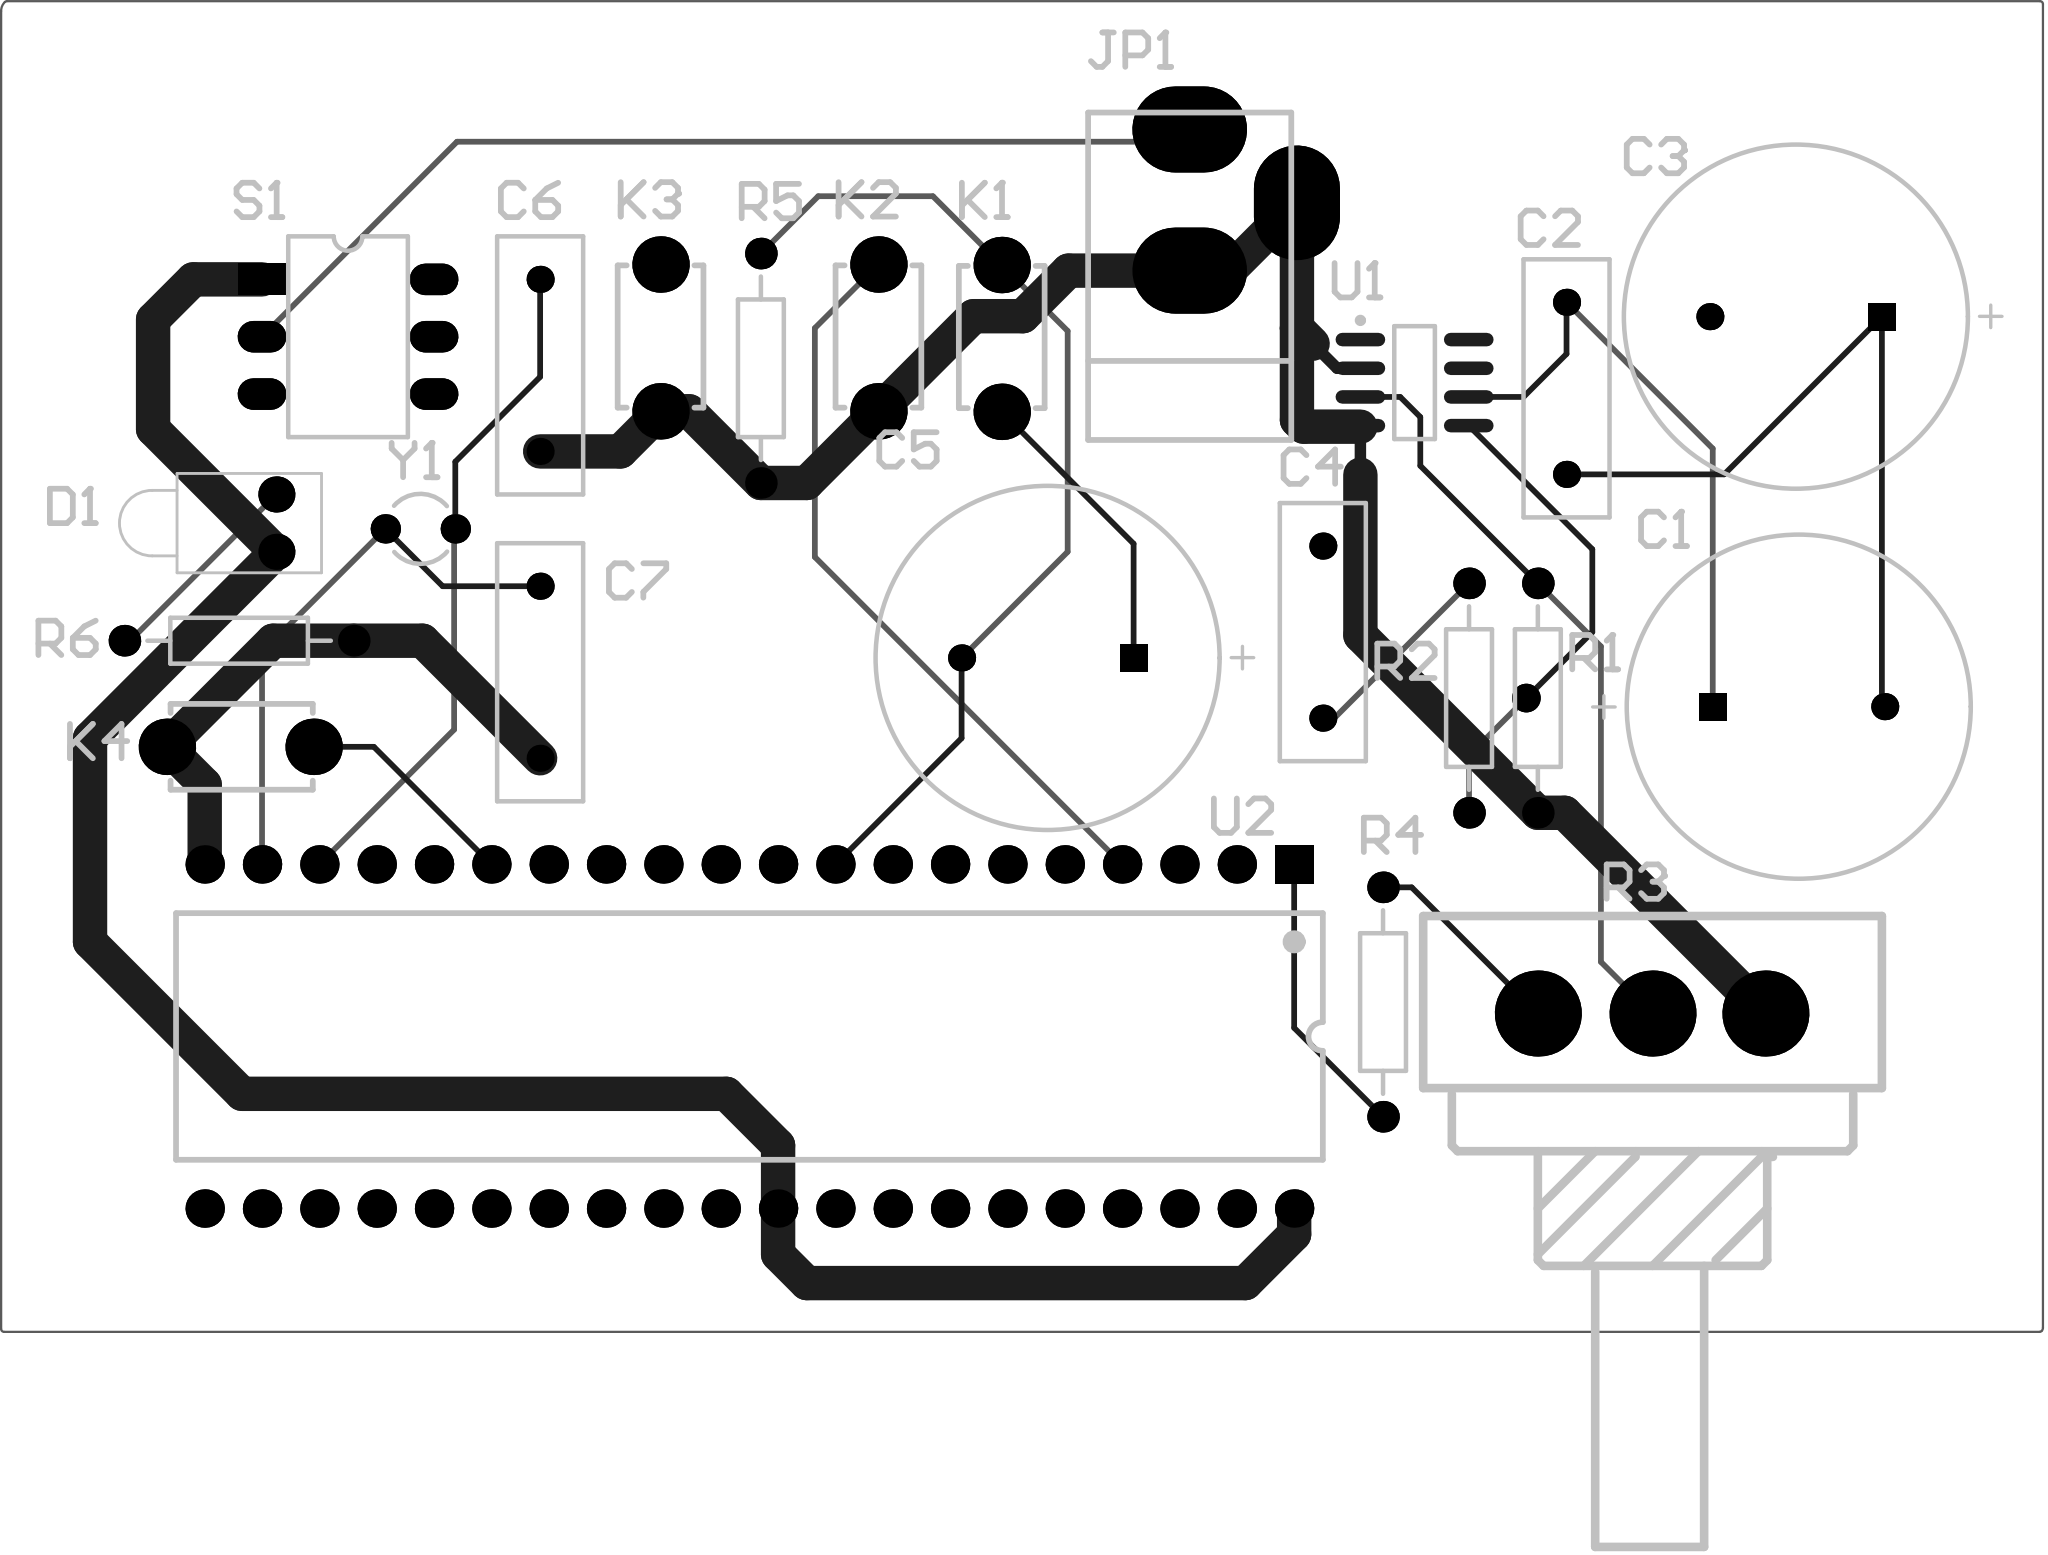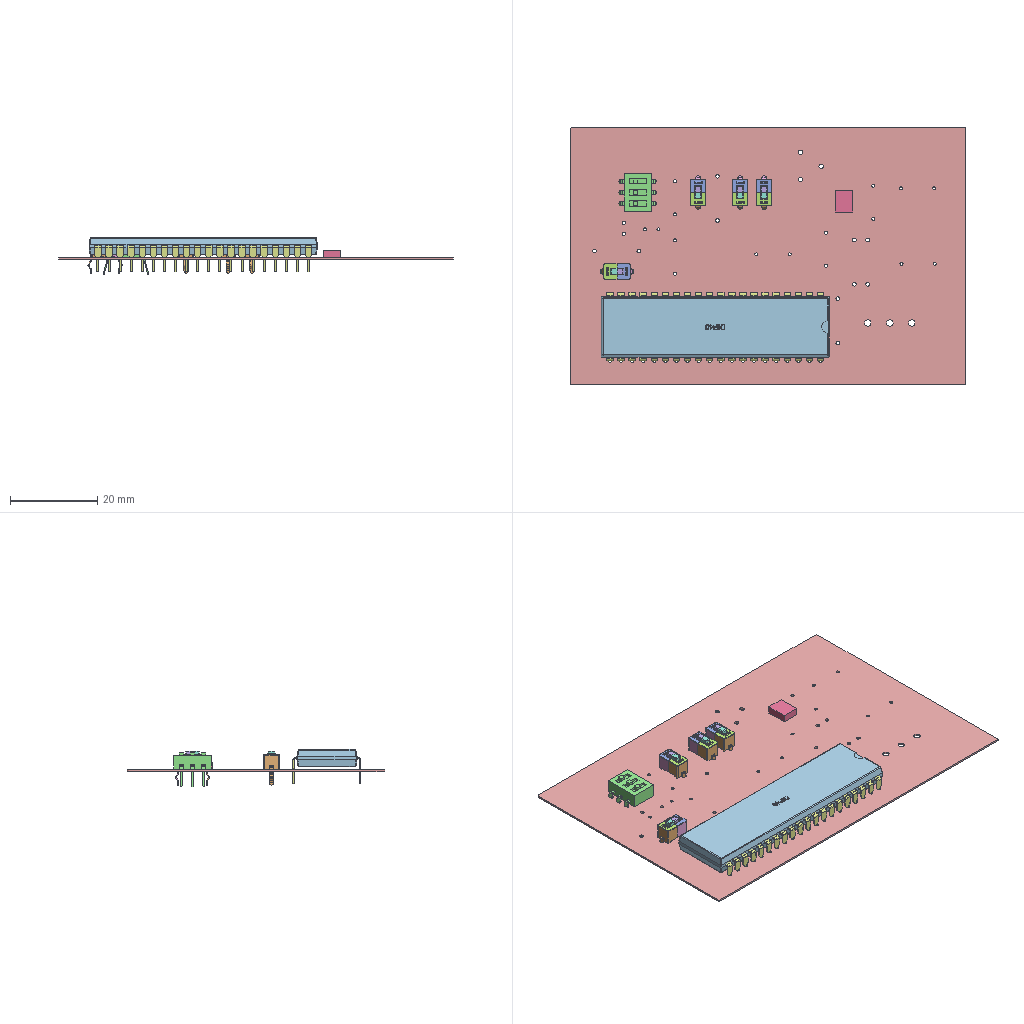Circuit board layout | Altium Designer | box 90.4 x 58.9 x 8.5 mm
Layer stack:
# Altium Designer layer stack of  (unit mm; dielectric type: 0 none, 1 core, 2 prepreg, 3 surface material)
index,name,kind,layer,copper_thickness_mm,dielectric_type,dielectric_thickness_mm,dielectric_material,dielectric_constant
0,Top Paste,other,,,,,,
1,Top Overlay,other,,,,,,
2,Top Solder,dielectric,,,3,0.0102,Solder Resist,3.5
3,Top Layer,copper,Top Layer,0.0356,,,,
4,Dielectric 1,dielectric,,,0,0.32,FR-4,4.8
5,Bottom Layer,copper,Bottom Layer,0.0356,,,,
6,Bottom Solder,dielectric,,,3,0.0102,Solder Resist,3.5
7,Bottom Overlay,other,,,,,,
8,Bottom Paste,other,,,,,,
# drill layer pairs: low layer,high layer
drill_pair,Top Layer,Bottom Layer
Part placement:
Designator,Comment,Layer,Footprint,Center-X(mm),Center-Y(mm),Rotation
C2,Cap,TopLayer,RAD-0.3,112.141,92.583,270
C1,Cap Pol1,TopLayer,RB7.6-15,122.428,78.486,180
C3,Cap Pol1,TopLayer,RB7.6-15,122.301,95.758,360
C4,Cap,TopLayer,RAD-0.3,101.346,81.788,90
C5,Cap Pol1,TopLayer,RB7.6-15,89.154,80.645,0
C6,Cap,TopLayer,RAD-0.3,66.675,93.599,90
C7,Cap,TopLayer,RAD-0.3,66.675,80.01,90
D1,LED1,TopLayer,LED-1,54.991,86.614,180
JP1,DC 5V,TopLayer,DC_POWER_JACK1,97.824,100.922,90
K1,KEY,TopLayer,DIP-3X6X4.3,87.122,94.794,90
K2,KEY,TopLayer,DIP-3X6X4.3,81.661,94.817,90
K3,KEY,TopLayer,DIP-3X6X4.3,72.009,94.817,90
K4,KEY,TopLayer,DIP-3X6X4.3,53.392,76.708,360
R3,Potentiometer,TopLayer,滑动变阻器,115.911,64.897,360
R4,Res2,TopLayer,AXIAL-0.4,104.013,65.405,90
R5,Res2,TopLayer,AXIAL-0.4,76.454,93.472,90
R6,Res2,TopLayer,AXIAL-0.4,53.34,81.407,360
S1,SW3-DIP6,TopLayer,DIP-Switch3,58.166,94.869,0
U1,LM386,TopLayer,M08A_N,105.41,92.837,0
U2,STC89C51,TopLayer,DIP40,75.946,63.881,270
Y1,XTAL,TopLayer,R38,61.367,86.36,90
R1,Res2,TopLayer,AXIAL-0.4,110.871,78.867,90
R2,Res2,TopLayer,AXIAL-0.4,107.823,78.867,90
Pad and via stacks:
# Altium Designer via and pad stacks of  (unit mm). Each distinct definition once, with the count of objects using it.
# via: kind,start_layer,end_layer,hole_mm,diameter_mm,mode(0 simple;1 top-mid-bottom;2 full stack),diameter_per_layer,count,example_net
# pad: kind,layer,hole_mm,hole_type(0 round;1 square;2 slot),plating,top_size,top_shape(1 round;2 rect;3 octagon;9 rounded rect),mid_size,bottom_size,mode,footprint,size_per_layer,count,example
pad,Multi-Layer,0.7,0,plated,1.2x1.2,1,1.2x1.2,1.2x1.2,0,RAD-0.3,,8,C2.1
pad,Multi-Layer,0.85,0,plated,1.4x1.4,1,1.4x1.4,1.4x1.4,0,AXIAL-0.4,,10,R6.2
pad,Multi-Layer,0.8,0,plated,1.6x1.6,1,1.6x1.6,1.6x1.6,0,LED-1,,2,D1.2
pad,Multi-Layer,0.7,0,plated,1.3x1.3,1,1.3x1.3,1.3x1.3,0,R38,,2,Y1.2
pad,Multi-Layer,1.2,0,plated,2.5x2.5,1,2.5x2.5,2.5x2.5,0,DIP-3X6X4.3,,8,K4.3
pad,Multi-Layer,0.9906,0,plated,2.159x1.397,2,2.159x1.397,2.159x1.397,0,DIP-Switch3,,1,S1.1
pad,Multi-Layer,0.9906,0,plated,2.159x1.397,1,2.159x1.397,2.159x1.397,0,DIP-Switch3,,5,S1.2
pad,Multi-Layer,0.7,0,plated,1.2x1.2,1,1.2x1.2,1.2x1.2,0,RB7.6-15,,3,C5.2
pad,Multi-Layer,0.7,0,plated,1.2x1.2,2,1.2x1.2,1.2x1.2,0,RB7.6-15,,3,C5.1
pad,Multi-Layer,1.016,0,plated,3.81x5.08,1,3.81x5.08,3.81x5.08,0,DC POWER JACK1,,2,JP1.1
pad,Multi-Layer,1.016,0,plated,5.08x3.81,1,5.08x3.81,5.08x3.81,0,DC POWER JACK1,,1,JP1.3
pad,Multi-Layer,0.8,0,plated,1.7x1.7,2,1.7x1.7,1.7x1.7,0,DIP40,,1,U2.1
pad,Multi-Layer,0.8,0,plated,1.7x1.7,1,1.7x1.7,1.7x1.7,0,DIP40,,39,U2.2
pad,Multi-Layer,1.5,0,plated,3.81x3.81,1,3.81x3.81,3.81x3.81,0,\u00BB\u00AC\u00B6\u00AF\u00B1\u00E4\u00D7\u00E8\u00C6\u00F7,,3,R3.1
pad,Top Layer,0,0,plated,0.6x2.2,1,0.6x2.2,0.6x2.2,0,M08A_N,,8,U1.1
via,Top Layer,Bottom Layer,0.7112,1.27,0,,1,NetR2_1
Design rules, without the lines most boards share:
# Altium Designer design rules of  (exported by Altium Designer, unit mm)
# columns: name | kind | enabled | priority | scope1 | scope2 | descriptor | typed fields (field=value)
Clearance | 0 | enabled | 1 | All | All | Clearance Constraint (Gap=0.254mm) (All),(All) | gap=0.254
PlaneConnect | 6 | enabled | 1 | All | All | Power Plane Connect Rule(Relief Connect )(Expansion=0.508mm) (Conductor Width=0.254mm) (Air Gap=0.254mm) (Entries=4) (All) | relief_conductor_width=0.254 relief_entries=4 relief_expansion=0.508
PlaneClearance | 12 | enabled | 1 | All | All | Power Plane Clearance (Clearance =0.508mm) (All) | clearance=0.508
PolygonConnect | 20 | enabled | 1 | All | All | Polygon Connect Rule(Relief Connect )(Conductor Width=0.254mm) (Relief Angle=90 Angle) (Entries=4) (Air Gap Width=0.254mm) (All),(All) | connect_style(0=relief,1=direct,2=none)=0 relief_conductor_width=0.254 relief_entries=4
Width | 2 | enabled | 1 | All | All | Width Constraint (Min=0.254mm) (Max=254mm) (Preferred=0.254mm) (All) |
RoutingCorners | 10 | enabled | 1 | All | All | Routing Corners (Style=45-Degree) (Min Setback=2.54mm) (Max Setback=2.54mm) (All) |
RoutingVias | 11 | enabled | 1 | All | All | Routing Via (MinHoleWidth=0.711mm) (MaxHoleWidth=0.711mm) (PreferredHoleWidth=0.711mm) (MinWidth=1.27mm) (MaxWidth=1.27mm) (PreferedWidth=1.27mm) (All) | via_min_hole=0.7112 via_max_hole=0.7112 via_preferred_diameter=1.27 via_preferred_hole=0.7112
PasteMaskExpansion | 14 | enabled | 1 | All | All | Paste Mask Expansion (Expansion =0mm) (All) | expansion=0
SolderMaskExpansion | 13 | enabled | 1 | All | All | Solder Mask Expansion (Expansion =0.102mm) (All) | expansion=0.1016
ComponentClearance | 24 | enabled | 1 | All | All | Component Clearance Constraint ( Horizontal Gap = 0.254mm, Vertical Gap = 0.254mm ) (All),(All)  | gap=0.254
Height | 50 | enabled | 1 | All | All | Height Constraint (Min=0mm) (Max=25.4mm) (Prefered=12.7mm) (All) | min_height=0 max_height=25.4
HoleSize | 42 | enabled | 1 | All | All | Hole Size Constraint (Min=0.025mm) (Max=2.54mm) (All) |
DiffPairsRouting | 51 | enabled | 1 | All | All | Differential Pairs Uncoupled Length using the Gap Constraints (Min=0.254mm) (Max=0.254mm) (Prefered=0.254mm)  and Width Constraints (Min=0.381mm) (Max=0.381mm) (Prefered=0.381mm) (All) |
HoleToHoleClearance | 52 | enabled | 1 | All | All | Hole To Hole Clearance (Gap=0.254mm) (All),(All) | gap=0.254
MinimumSolderMaskSliver | 53 | enabled | 1 | All | All | Minimum Solder Mask Sliver (Gap=0.254mm) (All),(All) |
SilkToSolderMaskClearance | 54 | enabled | 1 | IsPad | All | Silk To Solder Mask (Clearance=0.254mm) (IsPad),(All) |
SilkToSilkClearance | 55 | enabled | 1 | All | All | Silk to Silk (Clearance=0.254mm) (All),(All) |
NetAntennae | 56 | enabled | 1 | All | All | Net Antennae (Tolerance=0mm) (All) |
Classes set for this board:
# Altium Designer classes of  (member kind: 0 net, 1 component, 2 from-to, 3 pad, 4 layer, 5 differential pair, 6 design channel, 7 polygon, 8 structure, 9 xSignal)
# columns: class name | member kind | superclass | members
ZBW172 | 1 | no | B1; C1; C3; C4; C5; C6; C7; D1; JP1; K1; K2; K3; K4; R3; R4; R5; R6; S1; U1; U2; Y1;